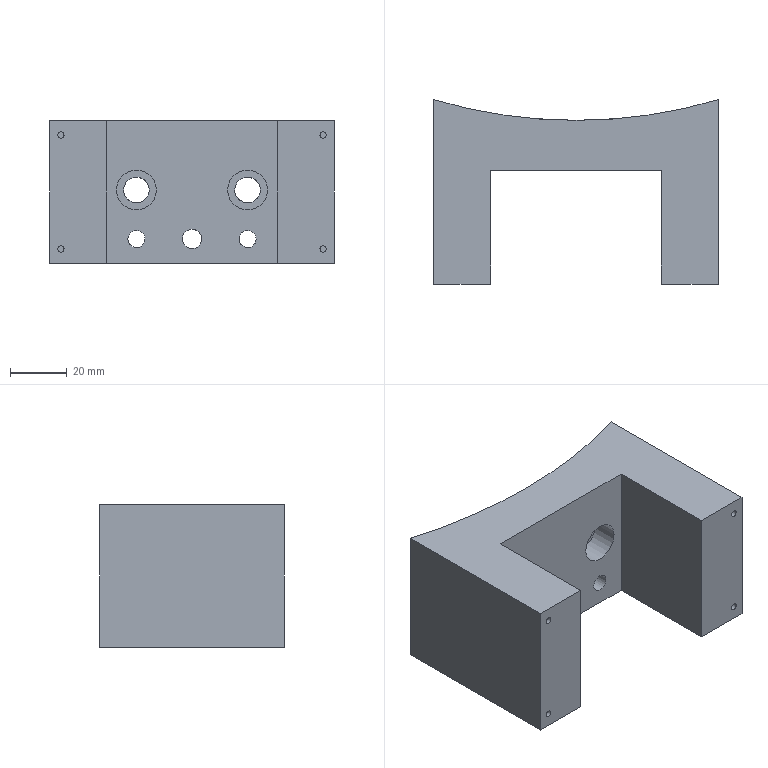NC program | NX | posted with a generic post | part box 100 x 64.77 x 50 mm
Lines 7595 to 7818 of 7818:
(DRILLING , TOOL : ZXZ)
N15188 T03 M6
N15190 G54
N15192 G17 G0 G90 X46. Y20. B0. C0. S3000 M3
N15194 G43 Z30. H3
N15196 G94 G81 G98 Z-1. F250. R3.
N15198 Y-20.
N15200 X19.5 Y-0.7 Z-41. R-37.
N15202 Y16.5
N15204 X0.
N15206 X-19.5
N15208 Y-0.7
N15210 X-46. Y-20. Z-1. R3.
N15212 Y20.
N15214 G80
N15216 G0 X-46. Y20. Z30.
N15218 M5
(DRILLING_COPY , TOOL : 2.2ZT)
N15220 T12 M6
N15222 G54
N15224 G17 G0 G90 X-46. Y-20. B0. C0. S2000 M3
N15226 G43 Z30. H12
N15228 G94 G83 G98 Z-11. F100. Q2. R3.
N15230 Y20.
N15232 X46.
N15234 Y-20.
N15236 G80
N15238 G0 X46. Y-20. Z30.
N15240 M5
(DRILLING_COPY_COPY , TOOL : 6.8ZT)
N15242 T16 M6
N15244 G54
N15246 G17 G0 G90 X0. Y16.5 B0. C0. S2000 M3
N15248 G43 Z30. H16
N15250 G94 G83 G98 Z-61.073 F180. Q2. R-37.
N15252 G80
N15254 G0 X0. Y16.5 Z30.
N15256 M5
(DRILLING_COPY_COPY_COPY , TOOL : 5.8ZT)
N15258 T15 M6
N15260 G54
N15262 G17 G0 G90 X-19.5 Y16.5 B0. C0. S2000 M3
N15264 G43 Z30. H15
N15266 G94 G83 G98 Z-62.188 F180. Q2. R-37.
N15268 X19.5
N15270 G80
N15272 G0 X19.5 Y16.5 Z30.
N15274 M5
(DRILLING_COPY_COPY_COPY_COPY , TOOL : 6.0JD)
N15276 T13 M6
N15278 G54
N15280 G17 G0 G90 X-19.5 Y16.5 B0. C0. S1000 M3
N15282 G43 Z30. H13
N15284 G94 G85 G98 Z-59.445 F50. R-37.
N15286 X19.5
N15288 G80
N15290 G0 X19.5 Y16.5 Z30.
N15292 M5
(DRILLING_COPY_1 , TOOL : 9.0ZT)
N15294 T09 M6
N15296 G54
N15298 G17 G0 G90 X-19.5 Y-0.7 B0. C0. S1000 M3
N15300 G43 Z30. H9
N15302 G94 G83 G98 Z-63.349 F200. Q2. R-37.
N15304 X19.5
N15306 G80
N15308 G0 X19.5 Y-0.7 Z30.
N15310 M5
(DRILLING_COPY_1_COPY , TOOL : 14.0UZ)
N15312 T14 M6
N15314 G54
N15316 G17 G0 G90 X-19.5 Y-0.7 B0. C0. S1000 M3
N15318 G43 Z30. H14
N15320 G94 G73 G98 Z-49. F150. Q3. R-37.
N15322 X19.5
N15324 G80
N15326 G0 X19.5 Y-0.7 Z30.
N15328 M5
(11 , TOOL : D10JING)
N15330 T11 M6
N15332 G54
N15334 G17 G0 G90 X24.081 Y-31.476 B0. C0. S5500 M3
N15336 G43 Z30. H11
N15338 Z-14.
N15340 G94 G1 Z-15. F1000.
N15342 X24.507 Y-31.227
N15344 G3 X25.003 Y-30.358 R1.
N15346 G1 X25.001 Y-29.912
N15348 Y-25.461
N15350 X25. Y-25.
N15352 Y24.554
N15354 X25.001 Y25.447
N15356 Y29.912
N15358 X25.003 Y30.358
N15360 G3 X24.507 Y31.227 R1.
N15362 G1 X24.081 Y31.476
N15364 Z-14.
N15366 G0 Y-31.476 Z-26.5
N15368 G1 Z-27.5
N15370 X24.507 Y-31.227
N15372 G3 X25.003 Y-30.358 R1.
N15374 G1 X25. Y-29.912
N15376 Y-25.
N15378 Y24.554
N15380 Y29.912
N15382 X25.003 Y30.358
N15384 G3 X24.507 Y31.227 R1.
N15386 G1 X24.081 Y31.476
N15388 Z-26.5
N15390 G0 X24.08 Y-31.476 Z-39.
N15392 G1 Z-40.
N15394 X24.507 Y-31.227
N15396 G3 X25.002 Y-30.358 R1.
N15398 G1 X25. Y-29.912
N15400 Y-25.
N15402 Y24.554
N15404 Y29.912
N15406 X25.002 Y30.358
N15408 G3 X24.507 Y31.227 R1.
N15410 G1 X24.081 Y31.476
N15412 Z-39.
N15414 G0 Z30.
N15416 X-24.079 Y31.469
N15418 Z-14.
N15420 G1 Z-15.
N15422 X-24.503 Y31.225
N15424 G3 X-25.002 Y30.358 R1.
N15426 G1 X-25. Y24.554
N15428 Y-25.
N15430 X-25.001 Y-25.461
N15432 Y-29.912
N15434 X-25.002 Y-30.358
N15436 G3 X-24.505 Y-31.226 R1.
N15438 G1 X-24.08 Y-31.473
N15440 Z-14.
N15442 G0 X-24.079 Y31.472 Z-26.5
N15444 G1 Z-27.5
N15446 X-24.503 Y31.225
N15448 G3 X-25.001 Y30.358 R1.
N15450 G1 X-25. Y29.912
N15452 Y24.554
N15454 Y-25.
N15456 Y-29.912
N15458 X-25.001 Y-30.358
N15460 G3 X-24.503 Y-31.225 R1.
N15462 G1 X-24.079 Y-31.472
N15464 Z-26.5
N15466 G0 X-24.078 Y31.469 Z-39.
N15468 G1 Z-40.
N15470 X-24.501 Y31.224
N15472 G3 X-25. Y30.358 R1.
N15474 G1 Y24.554
N15476 Y-25.
N15478 Y-30.358
N15480 G3 X-24.501 Y-31.224 R1.
N15482 G1 X-24.077 Y-31.469
N15484 Z-39.
N15486 G0 Z30.
(ZLEVEL_PROFILE_1_COPY_1_COPY , TOOL : D6A45)
N15488 T07 M6
N15490 G17 G43 G0 G90 X52.399 Y25.938 Z30. B0. C0. S7500 H7 M3
N15492 Z-0.5
N15494 G94 G1 Z-1.5 F1000.
N15496 X51.676 Y25.52
N15498 G3 X51.376 Y25.001 R0.6
N15500 G1 Y-25.001
N15502 G2 X50.001 Y-26.376 R1.375
N15504 G1 X29.999
N15506 G2 X28.624 Y-25.001 R1.375
N15508 G1 Y25.001
N15510 G2 X29.999 Y26.376 R1.375
N15512 G1 X50.001
N15514 G2 X51.376 Y25.001 R1.375
N15516 G3 X51.676 Y24.481 R0.6
N15518 G1 X52.576 Y23.962
N15520 Z-0.5
N15522 G0 Z30.
N15524 X-52.399 Y-25.938
N15526 Z-0.5
N15528 G1 Z-1.5
N15530 X-51.676 Y-25.52
N15532 G3 X-51.376 Y-25.001 R0.6
N15534 G1 Y25.001
N15536 G2 X-50.001 Y26.376 R1.375
N15538 G1 X-29.999
N15540 G2 X-28.624 Y25.001 R1.375
N15542 G1 Y-25.001
N15544 G2 X-29.999 Y-26.376 R1.375
N15546 G1 X-50.001
N15548 G2 X-51.376 Y-25.001 R1.375
N15550 G3 X-51.676 Y-24.481 R0.6
N15552 G1 X-52.576 Y-23.962
N15554 Z-0.5
N15556 G0 Z30.
(DRILLING_COPY_2 , TOOL : D6A45)
N15558 X-46. Y-20. S3000
N15560 G81 G98 Z-1.25 F250. R3.
N15562 Y20.
N15564 X46.
N15566 Y-20.
N15568 G80
N15570 G0 X46. Y-20. Z30.
N15572 M5
N15574 M2